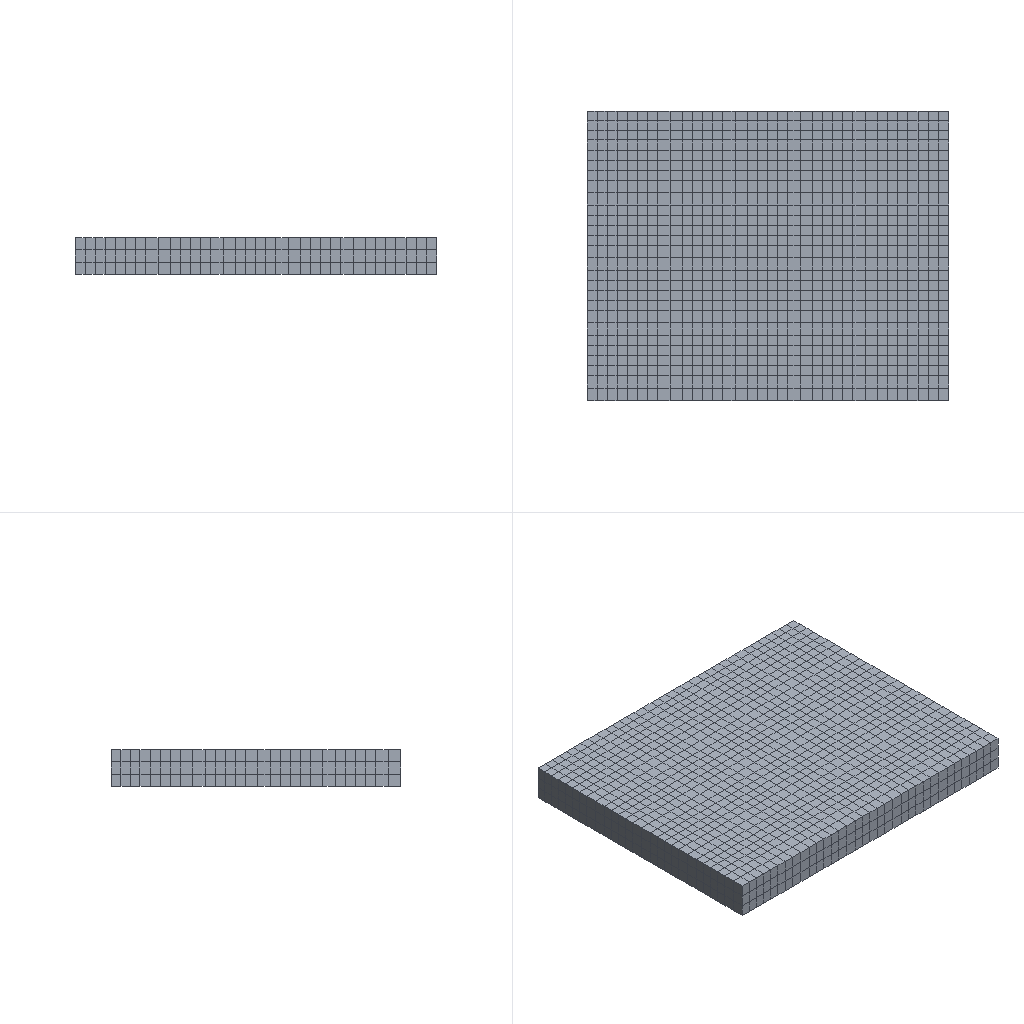Simulation study | abaqus
Set-up summary:
category,name,step,type,value,unit,region
solver,abaqus
solver,version,,,Abaqus/Standard 2020
units,not stated in the deck,,not stated
analysis,deck,,static,static
load_step,Step-1,Step-1,static
load_step,requested,,,1
mesh,nodes,,,4260
mesh,elements,,,3099
element_type,C3D8,,solid,2754
element_type,R3D3,,rigid,16
element_type,R3D4,,rigid,329
load,load commands in deck,,count,1
bc,support commands in deck,,count,7
material,COMPO,,in results
material,COMPO-XFEM,,in results
material,JITI,,in results
check,setup vs results,,match,"per instance, exact: element labels, types and connectivity; labels of the nodes the elements use; coordinates of those nodes at SINGLE_PRECISION in 2 of 2 instance(s)"
Abaqus input file, long lists of numbers shortened:
*Heading
** Job name: Job-2 Model name: Model-1-Copy
** Generated by: Abaqus/CAE 2020
*Preprint, echo=NO, model=NO, history=NO, contact=NO
**
** PARTS
**
*Part, name=ban
*Node
      1,   45.752,  -36.568,           0.
      2,   45.752,  -36.568,           5.
** (3918 more lines like these left out)
*Element, type=C3D8
 1,  258, 1383, 3093, 1377,    1,  241, 1373,  246
 2, 1383, 1384, 3094, 3093,  241,  242, 1374, 1373
** (2752 more lines like these left out)
*Nset, nset=Set-1
    1,    2,    5,    6,    9,   10,   11,   12,   13,   14,   15,   16,   17,   18,   19,   20
   21,   22,   23,   24,   25,   26,   27,   28,   29,   30,   31,   32,   50,   53,   57,   58
** (123 more lines like these left out)
*Elset, elset=Set-1, generate
 1795,  2754,     1
*Nset, nset=Set-2
    1,    2,    3,    4,    5,    6,    7,    8,    9,   10,   11,   12,   13,   14,   15,   16
   17,   18,   19,   20,   21,   22,   23,   24,   25,   26,   27,   28,   29,   30,   31,   32
** (198 more lines like these left out)
*Elset, elset=Set-2, generate
    1,  1794,     1
** Section: jiti
*Solid Section, elset=Set-2, material=jiti
,
*Orientation, name=Ori-1
1., 0., 0., 0., 1., 0.
1, 0.
** Section: Section-3
*Solid Section, elset=Set-1, orientation=Ori-1, material=compo-xfem
,
*End Part
**
*Part, name=crack
*End Part
**
*Part, name=sphere
*Node
      1,   1.113,   4.875,           0.
      2,   2.169,   4.505,           0.
** (337 more lines like these left out)
*Element, type=R3D3
 1, 336, 284, 248
 2, 157, 335,  19
** (14 more lines like these left out)
*Element, type=R3D4
 17,  68,  69,  64,  70
 18,  10,  11,  64,  69
** (327 more lines like these left out)
*Node
    340,           0., -3.061617e-16,           0.
*Nset, nset=sphere-RefPt_, internal
340,
*Elset, elset=sphere, generate
   1,  345,    1
*End Part
**
**
** ASSEMBLY
**
*Assembly, name=Assembly
**
*Instance, name=ban-1, part=ban
*End Instance
**
*Instance, name=sphere-1, part=sphere
    24.944,    -20.259,          -5.
*End Instance
**
*Instance, name=crack-1, part=crack
    24.944,    -22.759,           1.
    24.944,    -22.759,           1., 25.521, -22.181, 1.577,         120.
*End Instance
**
*Nset, nset=Set-1, instance=ban-1
    3,    4,    7,    8,   33,   34,   35,   36,   37,   38,   39,   40,   41,   42,   43,   44
   45,   46,   47,   48,   49,   51,   52,   54,   55,   56,   59,   60,   63,   64,   77,   78
** (29 more lines like these left out)
*Elset, elset=Set-1, instance=ban-1
    4,    5,    6,   10,   11,   12,   16,   17,   18,   22,   23,   24,  100,  101,  102,  106
  107,  108,  109,  110,  111,  112,  113,  114,  127,  128,  129,  130,  131,  132,  145,  146
** (21 more lines like these left out)
*Nset, nset=Set-3, instance=sphere-1
 340,
*Nset, nset=_PickedSet10, internal, instance=ban-1
    5,    6,   13,   14,   15,   16,   21,   22,   23,   24,   29,   30,   31,   32,   57,   58
   61,   62,   65,   66,   67,   68,   69,   70,   71,   72,   73,   74,   75,   76,   79,   80
** (119 more lines like these left out)
*Elset, elset=_PickedSet10, internal, instance=ban-1
  214,  215,  216,  217,  218,  219,  220,  221,  222,  223,  224,  225,  226,  227,  228,  229
  230,  231,  232,  233,  234,  235,  236,  237,  238,  239,  240,  241,  242,  243,  244,  245
** (81 more lines like these left out)
*Elset, elset=_m_Surf-3_SPOS, internal, instance=sphere-1, generate
   1,  345,    1
*Surface, type=ELEMENT, name=m_Surf-3
_m_Surf-3_SPOS, SPOS
*Elset, elset=_s_Surf-1_S6, internal, instance=ban-1
    1,    4,    7,   10,   13,   16,   19,   22,   25,   28,   31,   34,   37,   40,   43,   46
   49,   52,   55,   58,   61,   64,   67,   70,   97,  100,  103,  106,  109,  112,  115,  118
** (7 more lines like these left out)
*Elset, elset=_s_Surf-1_S3, internal, instance=ban-1
   73,   74,   79,   80,   85,   86,   91,   92,  151,  152,  157,  158,  163,  164,  946,  947
  948,  949,  958,  959,  960,  961,  970,  971,  972,  973,  982,  983,  984,  985,  994,  995
** (11 more lines like these left out)
*Elset, elset=_s_Surf-1_S1, internal, instance=ban-1
  187,  188,  189,  190,  191,  192,  193,  194,  195, 1827, 1828, 1829, 1830, 1831, 1832, 1833
 1834, 1835, 1836, 1837, 1838, 1839, 1840, 1841, 1842, 2019, 2020, 2021, 2022, 2023, 2024, 2025
** (6 more lines like these left out)
*Elset, elset=_s_Surf-1_S4, internal, instance=ban-1
  198,  201,  204,  207,  210,  213,  216,  219,  222,  225,  228,  231,  234,  237,  252,  255
  258,  261,  264,  267,  270,  273,  276,  279,  282,  285,  348,  351,  354,  357,  360,  363
** (9 more lines like these left out)
*Elset, elset=_s_Surf-1_S5, internal, instance=ban-1
  242,  243,  248,  249,  326,  327,  332,  333,  338,  339,  344,  345,  440,  441,  446,  447
  524,  525,  530,  531,  536,  537,  542,  543,  638,  639,  644,  645,  770,  771,  776,  777
** (3 more lines like these left out)
*Elset, elset=_s_Surf-1_S2, internal, instance=ban-1
 1843, 1844, 1845, 1846, 1847, 1848, 1849, 1850, 1851, 1852, 1853, 1854, 1855, 1856, 1857, 1858
 1891, 1892, 1893, 1894, 1895, 1896, 1897, 1898, 1899, 1900, 1901, 1902, 1903, 1904, 1905, 1906
** (11 more lines like these left out)
*Surface, type=ELEMENT, name=s_Surf-1
_s_Surf-1_S6, S6
_s_Surf-1_S3, S3
_s_Surf-1_S4, S4
_s_Surf-1_S2, S2
_s_Surf-1_S1, S1
_s_Surf-1_S5, S5
*Rigid Body, ref node=sphere-1.sphere-RefPt_, elset=sphere-1.sphere
*Enrichment, name=Crack-1, type=PROPAGATION CRACK, elset=_PickedSet10
*End Assembly
*Amplitude, name=Amp-1
             0.,              0.,              1.,              1.
**
** MATERIALS
**
*Material, name=compo
*Damage Initiation, criterion=HASHIN
297., 326.8, 367.8, 48.38,  21.7,  65.1
*Damage Evolution, type=ENERGY
 0.3, 0.1, 0.7, 0.2
*Damage Stabilization
0.001,0.001,0.001,0.001
*Elastic, type=ENGINEERING CONSTANTS
23420.,22860.,40900.,  0.29,   0.3,   0.3, 2130.,11830.
21700.,
*Material, name=compo-xfem
*Damage Initiation, criterion=MAXPS
1.,
*Damage Evolution, type=DISPLACEMENT
 1e-06,
*Damage Stabilization
0.001
*Elastic, type=ENGINEERING CONSTANTS
23420.,22860.,40900.,  0.29,   0.3,   0.3, 2130.,11830.
21700.,
*Material, name=jiti
*Damage Initiation, criterion=QUADE
 0.001, 0.001, 0.001
*Damage Evolution, type=DISPLACEMENT
 0.0001,
*Damage Stabilization
0.001
*Elastic
2000., 0.3
**
** INTERACTION PROPERTIES
**
*Surface Interaction, name=IntProp-1
1.,
*Friction, slip tolerance=0.005
 0.3,
*Surface Behavior, pressure-overclosure=HARD
*Surface Interaction, name=IntProp-2
1.,
*Initial Conditions, type=ENRICHMENT
ban-1.552, 1,Crack-1, -1.404, 0.4192
ban-1.552, 2,Crack-1, -1.404, -0.6288
ban-1.552, 3,Crack-1, -1.404, -1.
ban-1.552, 4,Crack-1, -1.404, 0.6667
ban-1.552, 5,Crack-1, 1e-06, 0.4192
ban-1.552, 6,Crack-1, 1e-06, -0.6288
ban-1.552, 7,Crack-1, 1e-06, -1.
ban-1.552, 8,Crack-1, 1e-06, 0.6667
ban-1.257, 1,Crack-1, -1.404, 1.511
ban-1.257, 2,Crack-1, -1.404, 0.4192
ban-1.257, 3,Crack-1, 1e-06, 0.4192
ban-1.257, 4,Crack-1, 1e-06, 1.511
ban-1.257, 5,Crack-1, -1.404, 0.4631
ban-1.257, 6,Crack-1, -1.404, -0.6288
ban-1.257, 7,Crack-1, 1e-06, -0.6288
ban-1.257, 8,Crack-1, 1e-06, 0.4631
ban-1.555, 1,Crack-1, -1.404, 0.6667
ban-1.555, 2,Crack-1, -1.404, -1.
ban-1.555, 3,Crack-1, -1.404, -0.6288
ban-1.555, 4,Crack-1, -1.404, 0.4192
ban-1.555, 5,Crack-1, 1e-06, 0.6667
ban-1.555, 6,Crack-1, 1e-06, -1.
ban-1.555, 7,Crack-1, 1e-06, -0.6288
ban-1.555, 8,Crack-1, 1e-06, 0.4192
ban-1.209, 1,Crack-1, -1.404, 0.4192
ban-1.209, 2,Crack-1, -1.404, 1.511
ban-1.209, 3,Crack-1, 1e-06, 1.511
ban-1.209, 4,Crack-1, 1e-06, 0.4192
ban-1.209, 5,Crack-1, -1.404, -0.6288
ban-1.209, 6,Crack-1, -1.404, 0.4631
ban-1.209, 7,Crack-1, 1e-06, 0.4631
ban-1.209, 8,Crack-1, 1e-06, -0.6288
**
** INTERACTIONS
**
** Interaction: Int-1
*Contact Pair, interaction=IntProp-1, type=SURFACE TO SURFACE
s_Surf-1, m_Surf-3
** ----------------------------------------------------------------
**
** STEP: Step-1
**
*Step, name=Step-1, nlgeom=YES, inc=1000
*Static, stabilize=0.0002, allsdtol=0.05, continue=NO
0.001, 1., 1e-05, 1.
**
** BOUNDARY CONDITIONS
**
** Name: BC-1 Type: 对称/反对称/完全固定
*Boundary
Set-1, ENCASTRE
** Name: [REDACTED] : Displacement/rotation angle
*Boundary, amplitude=Amp-1
Set-3, 1, 1
Set-3, 2, 2
Set-3, 3, 3, 1.
Set-3, 4, 4
Set-3, 5, 5
Set-3, 6, 6
**
** OUTPUT REQUESTS
**
*Restart, write, frequency=0
**
** FIELD OUTPUT: F-Output-1
**
*Output, field
*Node Output
CF, PHILSM, PSILSM, RF, U, V
*Element Output, directions=YES
E, ENRRTXFEM, LE, LOADSXFEM, MISES, MISESMAX, PE, PEEQ, PEMAG, S, SDEG, STATUS, STATUSXFEM
*Contact Output
CDISP, CSTRESS
**
** HISTORY OUTPUT: H-Output-1
**
*Output, history, variable=PRESELECT
*End Step
Results summary:
result,step,,partial,increments=187 time=0.2024/1.0
result,analysis,,,static
result,last_loadstep,,,1
result,primary field,,,U
result,reaction total,,FX,1.065,model units
result,reaction total,,FY,-0.4334,model units
result,reaction total,,FZ,0.9512,model units